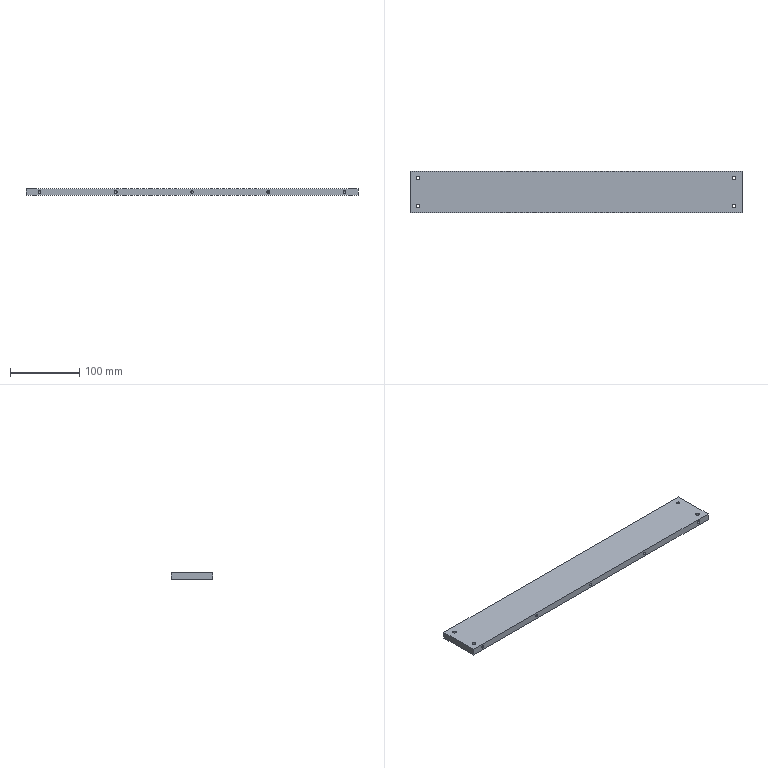Part | SolidWorks | features HoleWzd 3, Extrusion 1 | 1 solid | 46 faces | box 479 x 60 x 10 mm | volume 285459 mm3 | cylinder 24 | cone 16 | plane 6 | commonest cylinder face diameters 4.2 x10 5 x8 3.3 x6
STEP:
#1=CARTESIAN_POINT('',(0.,49.9,-1.65));
#2=VERTEX_POINT('',#1);
#3=CARTESIAN_POINT('',(0.,49.9,1.65));
#4=VERTEX_POINT('',#3);
#5=CARTESIAN_POINT('',(0.,49.9,0.));
#6=DIRECTION('',(0.,1.,0.));
#7=DIRECTION('',(0.,0.,1.));
#8=AXIS2_PLACEMENT_3D('',#5,#6,#7);
#9=CIRCLE('',#8,1.65);
#10=EDGE_CURVE('',#2,#4,#9,.T.);
#11=ORIENTED_EDGE('',*,*,#10,.F.);
#12=CARTESIAN_POINT('',(0.,60.,-1.65));
#13=VERTEX_POINT('',#12);
#14=CARTESIAN_POINT('',(0.,60.,-1.65));
#15=DIRECTION('',(0.,1.,0.));
#16=VECTOR('',#15,1000.);
#17=LINE('',#14,#16);
#18=EDGE_CURVE('',#2,#13,#17,.T.);
#19=ORIENTED_EDGE('',*,*,#18,.T.);
#20=CARTESIAN_POINT('',(0.,60.,1.65));
#21=VERTEX_POINT('',#20);
#22=CARTESIAN_POINT('',(0.,60.,0.));
#23=DIRECTION('',(0.,1.,0.));
#24=DIRECTION('',(0.,0.,1.));
#25=AXIS2_PLACEMENT_3D('',#22,#23,#24);
#26=CIRCLE('',#25,1.65);
#27=EDGE_CURVE('',#13,#21,#26,.T.);
#28=ORIENTED_EDGE('',*,*,#27,.T.);
#29=CARTESIAN_POINT('',(0.,60.,1.65));
#30=DIRECTION('',(0.,1.,0.));
#31=VECTOR('',#30,1000.);
#32=LINE('',#29,#31);
#33=EDGE_CURVE('',#4,#21,#32,.T.);
#34=ORIENTED_EDGE('',*,*,#33,.F.);
#35=EDGE_LOOP('',(#11,#19,#28,#34));
#36=FACE_OUTER_BOUND('',#35,.T.);
#37=CARTESIAN_POINT('',(0.,60.,0.));
#38=DIRECTION('',(0.,1.,0.));
#39=DIRECTION('',(0.,0.,1.));
#40=AXIS2_PLACEMENT_3D('',#37,#38,#39);
#41=CYLINDRICAL_SURFACE('',#40,1.65);
#42=ADVANCED_FACE('',(#36),#41,.F.);
#43=CARTESIAN_POINT('',(0.,48.909,0.));
#44=VERTEX_POINT('',#43);
#45=CARTESIAN_POINT('',(0.,49.9,1.65));
#46=DIRECTION('',(0.,0.515,0.8572));
#47=VECTOR('',#46,1000.);
#48=LINE('',#45,#47);
#49=EDGE_CURVE('',#44,#4,#48,.T.);
#50=ORIENTED_EDGE('',*,*,#49,.F.);
#51=CARTESIAN_POINT('',(0.,49.9,-1.65));
#52=DIRECTION('',(0.,0.515,-0.8572));
#53=VECTOR('',#52,1000.);
#54=LINE('',#51,#53);
#55=EDGE_CURVE('',#44,#2,#54,.T.);
#56=ORIENTED_EDGE('',*,*,#55,.T.);
#57=ORIENTED_EDGE('',*,*,#10,.T.);
#58=EDGE_LOOP('',(#50,#56,#57));
#59=FACE_OUTER_BOUND('',#58,.T.);
#60=CARTESIAN_POINT('',(0.,49.9,0.));
#61=DIRECTION('',(0.,1.,0.));
#62=DIRECTION('',(0.,0.,1.));
#63=AXIS2_PLACEMENT_3D('',#60,#61,#62);
#64=CONICAL_SURFACE('',#63,1.65,1.03);
#65=ADVANCED_FACE('',(#59),#64,.F.);
#66=CARTESIAN_POINT('',(-160.,49.9,-1.65));
#67=VERTEX_POINT('',#66);
#68=CARTESIAN_POINT('',(-160.,49.9,1.65));
#69=VERTEX_POINT('',#68);
#70=CARTESIAN_POINT('',(-160.,49.9,0.));
#71=DIRECTION('',(0.,1.,0.));
#72=DIRECTION('',(0.,0.,1.));
#73=AXIS2_PLACEMENT_3D('',#70,#71,#72);
#74=CIRCLE('',#73,1.65);
#75=EDGE_CURVE('',#67,#69,#74,.T.);
#76=ORIENTED_EDGE('',*,*,#75,.F.);
#77=CARTESIAN_POINT('',(-160.,60.,-1.65));
#78=VERTEX_POINT('',#77);
#79=CARTESIAN_POINT('',(-160.,60.,-1.65));
#80=DIRECTION('',(0.,1.,0.));
#81=VECTOR('',#80,1000.);
#82=LINE('',#79,#81);
#83=EDGE_CURVE('',#67,#78,#82,.T.);
#84=ORIENTED_EDGE('',*,*,#83,.T.);
#85=CARTESIAN_POINT('',(-160.,60.,1.65));
#86=VERTEX_POINT('',#85);
#87=CARTESIAN_POINT('',(-160.,60.,0.));
#88=DIRECTION('',(0.,1.,0.));
#89=DIRECTION('',(0.,0.,1.));
#90=AXIS2_PLACEMENT_3D('',#87,#88,#89);
#91=CIRCLE('',#90,1.65);
#92=EDGE_CURVE('',#78,#86,#91,.T.);
#93=ORIENTED_EDGE('',*,*,#92,.T.);
#94=CARTESIAN_POINT('',(-160.,60.,1.65));
#95=DIRECTION('',(0.,1.,0.));
#96=VECTOR('',#95,1000.);
#97=LINE('',#94,#96);
#98=EDGE_CURVE('',#69,#86,#97,.T.);
#99=ORIENTED_EDGE('',*,*,#98,.F.);
#100=EDGE_LOOP('',(#76,#84,#93,#99));
#101=FACE_OUTER_BOUND('',#100,.T.);
#102=CARTESIAN_POINT('',(-160.,60.,0.));
#103=DIRECTION('',(0.,1.,0.));
#104=DIRECTION('',(0.,0.,1.));
#105=AXIS2_PLACEMENT_3D('',#102,#103,#104);
#106=CYLINDRICAL_SURFACE('',#105,1.65);
#107=ADVANCED_FACE('',(#101),#106,.F.);
#108=CARTESIAN_POINT('',(-160.,48.909,0.));
#109=VERTEX_POINT('',#108);
#110=CARTESIAN_POINT('',(-160.,49.9,1.65));
#111=DIRECTION('',(0.,0.515,0.8572));
#112=VECTOR('',#111,1000.);
#113=LINE('',#110,#112);
#114=EDGE_CURVE('',#109,#69,#113,.T.);
#115=ORIENTED_EDGE('',*,*,#114,.F.);
#116=CARTESIAN_POINT('',(-160.,49.9,-1.65));
#117=DIRECTION('',(0.,0.515,-0.8572));
#118=VECTOR('',#117,1000.);
#119=LINE('',#116,#118);
#120=EDGE_CURVE('',#109,#67,#119,.T.);
#121=ORIENTED_EDGE('',*,*,#120,.T.);
#122=ORIENTED_EDGE('',*,*,#75,.T.);
#123=EDGE_LOOP('',(#115,#121,#122));
#124=FACE_OUTER_BOUND('',#123,.T.);
#125=CARTESIAN_POINT('',(-160.,49.9,0.));
#126=DIRECTION('',(0.,1.,0.));
#127=DIRECTION('',(0.,0.,1.));
#128=AXIS2_PLACEMENT_3D('',#125,#126,#127);
#129=CONICAL_SURFACE('',#128,1.65,1.03);
#130=ADVANCED_FACE('',(#124),#129,.F.);
#131=CARTESIAN_POINT('',(160.,49.9,-1.65));
#132=VERTEX_POINT('',#131);
#133=CARTESIAN_POINT('',(160.,49.9,1.65));
#134=VERTEX_POINT('',#133);
#135=CARTESIAN_POINT('',(160.,49.9,0.));
#136=DIRECTION('',(0.,1.,0.));
#137=DIRECTION('',(0.,0.,1.));
#138=AXIS2_PLACEMENT_3D('',#135,#136,#137);
#139=CIRCLE('',#138,1.65);
#140=EDGE_CURVE('',#132,#134,#139,.T.);
#141=ORIENTED_EDGE('',*,*,#140,.F.);
#142=CARTESIAN_POINT('',(160.,60.,-1.65));
#143=VERTEX_POINT('',#142);
#144=CARTESIAN_POINT('',(160.,60.,-1.65));
#145=DIRECTION('',(0.,1.,0.));
#146=VECTOR('',#145,1000.);
#147=LINE('',#144,#146);
#148=EDGE_CURVE('',#132,#143,#147,.T.);
#149=ORIENTED_EDGE('',*,*,#148,.T.);
#150=CARTESIAN_POINT('',(160.,60.,1.65));
#151=VERTEX_POINT('',#150);
#152=CARTESIAN_POINT('',(160.,60.,0.));
#153=DIRECTION('',(0.,1.,0.));
#154=DIRECTION('',(0.,0.,1.));
#155=AXIS2_PLACEMENT_3D('',#152,#153,#154);
#156=CIRCLE('',#155,1.65);
#157=EDGE_CURVE('',#143,#151,#156,.T.);
#158=ORIENTED_EDGE('',*,*,#157,.T.);
#159=CARTESIAN_POINT('',(160.,60.,1.65));
#160=DIRECTION('',(0.,1.,0.));
#161=VECTOR('',#160,1000.);
#162=LINE('',#159,#161);
#163=EDGE_CURVE('',#134,#151,#162,.T.);
#164=ORIENTED_EDGE('',*,*,#163,.F.);
#165=EDGE_LOOP('',(#141,#149,#158,#164));
#166=FACE_OUTER_BOUND('',#165,.T.);
#167=CARTESIAN_POINT('',(160.,60.,0.));
#168=DIRECTION('',(0.,1.,0.));
#169=DIRECTION('',(0.,0.,1.));
#170=AXIS2_PLACEMENT_3D('',#167,#168,#169);
#171=CYLINDRICAL_SURFACE('',#170,1.65);
#172=ADVANCED_FACE('',(#166),#171,.F.);
#173=CARTESIAN_POINT('',(160.,48.909,0.));
#174=VERTEX_POINT('',#173);
#175=CARTESIAN_POINT('',(160.,49.9,1.65));
#176=DIRECTION('',(0.,0.515,0.8572));
#177=VECTOR('',#176,1000.);
#178=LINE('',#175,#177);
#179=EDGE_CURVE('',#174,#134,#178,.T.);
#180=ORIENTED_EDGE('',*,*,#179,.F.);
#181=CARTESIAN_POINT('',(160.,49.9,-1.65));
#182=DIRECTION('',(0.,0.515,-0.8572));
#183=VECTOR('',#182,1000.);
#184=LINE('',#181,#183);
#185=EDGE_CURVE('',#174,#132,#184,.T.);
#186=ORIENTED_EDGE('',*,*,#185,.T.);
#187=ORIENTED_EDGE('',*,*,#140,.T.);
#188=EDGE_LOOP('',(#180,#186,#187));
#189=FACE_OUTER_BOUND('',#188,.T.);
#190=CARTESIAN_POINT('',(160.,49.9,0.));
#191=DIRECTION('',(0.,1.,0.));
#192=DIRECTION('',(0.,0.,1.));
#193=AXIS2_PLACEMENT_3D('',#190,#191,#192);
#194=CONICAL_SURFACE('',#193,1.65,1.03);
#195=ADVANCED_FACE('',(#189),#194,.F.);
#196=CARTESIAN_POINT('',(-225.5,50.,5.));
#197=VERTEX_POINT('',#196);
#198=CARTESIAN_POINT('',(-230.5,50.,5.));
#199=VERTEX_POINT('',#198);
#200=CARTESIAN_POINT('',(-228.,50.,5.));
#201=DIRECTION('',(0.,0.,-1.));
#202=DIRECTION('',(-1.,0.,0.));
#203=AXIS2_PLACEMENT_3D('',#200,#201,#202);
#204=CIRCLE('',#203,2.5);
#205=EDGE_CURVE('',#197,#199,#204,.T.);
#206=ORIENTED_EDGE('',*,*,#205,.F.);
#207=CARTESIAN_POINT('',(-225.5,50.,-5.));
#208=VERTEX_POINT('',#207);
#209=CARTESIAN_POINT('',(-225.5,50.,-5.));
#210=DIRECTION('',(0.,0.,-1.));
#211=VECTOR('',#210,1000.);
#212=LINE('',#209,#211);
#213=EDGE_CURVE('',#197,#208,#212,.T.);
#214=ORIENTED_EDGE('',*,*,#213,.T.);
#215=CARTESIAN_POINT('',(-230.5,50.,-5.));
#216=VERTEX_POINT('',#215);
#217=CARTESIAN_POINT('',(-228.,50.,-5.));
#218=DIRECTION('',(0.,0.,-1.));
#219=DIRECTION('',(-1.,0.,0.));
#220=AXIS2_PLACEMENT_3D('',#217,#218,#219);
#221=CIRCLE('',#220,2.5);
#222=EDGE_CURVE('',#208,#216,#221,.T.);
#223=ORIENTED_EDGE('',*,*,#222,.T.);
#224=CARTESIAN_POINT('',(-230.5,50.,-5.));
#225=DIRECTION('',(0.,0.,-1.));
#226=VECTOR('',#225,1000.);
#227=LINE('',#224,#226);
#228=EDGE_CURVE('',#199,#216,#227,.T.);
#229=ORIENTED_EDGE('',*,*,#228,.F.);
#230=EDGE_LOOP('',(#206,#214,#223,#229));
#231=FACE_OUTER_BOUND('',#230,.T.);
#232=CARTESIAN_POINT('',(-228.,50.,-5.));
#233=DIRECTION('',(0.,0.,-1.));
#234=DIRECTION('',(-1.,0.,0.));
#235=AXIS2_PLACEMENT_3D('',#232,#233,#234);
#236=CYLINDRICAL_SURFACE('',#235,2.5);
#237=ADVANCED_FACE('',(#231),#236,.F.);
#238=CARTESIAN_POINT('',(-225.5,10.,5.));
#239=VERTEX_POINT('',#238);
#240=CARTESIAN_POINT('',(-230.5,10.,5.));
#241=VERTEX_POINT('',#240);
#242=CARTESIAN_POINT('',(-228.,10.,5.));
#243=DIRECTION('',(0.,0.,-1.));
#244=DIRECTION('',(-1.,0.,0.));
#245=AXIS2_PLACEMENT_3D('',#242,#243,#244);
#246=CIRCLE('',#245,2.5);
#247=EDGE_CURVE('',#239,#241,#246,.T.);
#248=ORIENTED_EDGE('',*,*,#247,.F.);
#249=CARTESIAN_POINT('',(-225.5,10.,-5.));
#250=VERTEX_POINT('',#249);
#251=CARTESIAN_POINT('',(-225.5,10.,-5.));
#252=DIRECTION('',(0.,0.,-1.));
#253=VECTOR('',#252,1000.);
#254=LINE('',#251,#253);
#255=EDGE_CURVE('',#239,#250,#254,.T.);
#256=ORIENTED_EDGE('',*,*,#255,.T.);
#257=CARTESIAN_POINT('',(-230.5,10.,-5.));
#258=VERTEX_POINT('',#257);
#259=CARTESIAN_POINT('',(-228.,10.,-5.));
#260=DIRECTION('',(0.,0.,-1.));
#261=DIRECTION('',(-1.,0.,0.));
#262=AXIS2_PLACEMENT_3D('',#259,#260,#261);
#263=CIRCLE('',#262,2.5);
#264=EDGE_CURVE('',#250,#258,#263,.T.);
#265=ORIENTED_EDGE('',*,*,#264,.T.);
#266=CARTESIAN_POINT('',(-230.5,10.,-5.));
#267=DIRECTION('',(0.,0.,-1.));
#268=VECTOR('',#267,1000.);
#269=LINE('',#266,#268);
#270=EDGE_CURVE('',#241,#258,#269,.T.);
#271=ORIENTED_EDGE('',*,*,#270,.F.);
#272=EDGE_LOOP('',(#248,#256,#265,#271));
#273=FACE_OUTER_BOUND('',#272,.T.);
#274=CARTESIAN_POINT('',(-228.,10.,-5.));
#275=DIRECTION('',(0.,0.,-1.));
#276=DIRECTION('',(-1.,0.,0.));
#277=AXIS2_PLACEMENT_3D('',#274,#275,#276);
#278=CYLINDRICAL_SURFACE('',#277,2.5);
#279=ADVANCED_FACE('',(#273),#278,.F.);
#280=CARTESIAN_POINT('',(230.5,10.,5.));
#281=VERTEX_POINT('',#280);
#282=CARTESIAN_POINT('',(225.5,10.,5.));
#283=VERTEX_POINT('',#282);
#284=CARTESIAN_POINT('',(228.,10.,5.));
#285=DIRECTION('',(0.,0.,-1.));
#286=DIRECTION('',(-1.,0.,0.));
#287=AXIS2_PLACEMENT_3D('',#284,#285,#286);
#288=CIRCLE('',#287,2.5);
#289=EDGE_CURVE('',#281,#283,#288,.T.);
#290=ORIENTED_EDGE('',*,*,#289,.F.);
#291=CARTESIAN_POINT('',(230.5,10.,-5.));
#292=VERTEX_POINT('',#291);
#293=CARTESIAN_POINT('',(230.5,10.,-5.));
#294=DIRECTION('',(0.,0.,-1.));
#295=VECTOR('',#294,1000.);
#296=LINE('',#293,#295);
#297=EDGE_CURVE('',#281,#292,#296,.T.);
#298=ORIENTED_EDGE('',*,*,#297,.T.);
#299=CARTESIAN_POINT('',(225.5,10.,-5.));
#300=VERTEX_POINT('',#299);
#301=CARTESIAN_POINT('',(228.,10.,-5.));
#302=DIRECTION('',(0.,0.,-1.));
#303=DIRECTION('',(-1.,0.,0.));
#304=AXIS2_PLACEMENT_3D('',#301,#302,#303);
#305=CIRCLE('',#304,2.5);
#306=EDGE_CURVE('',#292,#300,#305,.T.);
#307=ORIENTED_EDGE('',*,*,#306,.T.);
#308=CARTESIAN_POINT('',(225.5,10.,-5.));
#309=DIRECTION('',(0.,0.,-1.));
#310=VECTOR('',#309,1000.);
#311=LINE('',#308,#310);
#312=EDGE_CURVE('',#283,#300,#311,.T.);
#313=ORIENTED_EDGE('',*,*,#312,.F.);
#314=EDGE_LOOP('',(#290,#298,#307,#313));
#315=FACE_OUTER_BOUND('',#314,.T.);
#316=CARTESIAN_POINT('',(228.,10.,-5.));
#317=DIRECTION('',(0.,0.,-1.));
#318=DIRECTION('',(-1.,0.,0.));
#319=AXIS2_PLACEMENT_3D('',#316,#317,#318);
#320=CYLINDRICAL_SURFACE('',#319,2.5);
#321=ADVANCED_FACE('',(#315),#320,.F.);
#322=CARTESIAN_POINT('',(230.5,50.,5.));
#323=VERTEX_POINT('',#322);
#324=CARTESIAN_POINT('',(225.5,50.,5.));
#325=VERTEX_POINT('',#324);
#326=CARTESIAN_POINT('',(228.,50.,5.));
#327=DIRECTION('',(0.,0.,-1.));
#328=DIRECTION('',(-1.,0.,0.));
#329=AXIS2_PLACEMENT_3D('',#326,#327,#328);
#330=CIRCLE('',#329,2.5);
#331=EDGE_CURVE('',#323,#325,#330,.T.);
#332=ORIENTED_EDGE('',*,*,#331,.F.);
#333=CARTESIAN_POINT('',(230.5,50.,-5.));
#334=VERTEX_POINT('',#333);
#335=CARTESIAN_POINT('',(230.5,50.,-5.));
#336=DIRECTION('',(0.,0.,-1.));
#337=VECTOR('',#336,1000.);
#338=LINE('',#335,#337);
#339=EDGE_CURVE('',#323,#334,#338,.T.);
#340=ORIENTED_EDGE('',*,*,#339,.T.);
#341=CARTESIAN_POINT('',(225.5,50.,-5.));
#342=VERTEX_POINT('',#341);
#343=CARTESIAN_POINT('',(228.,50.,-5.));
#344=DIRECTION('',(0.,0.,-1.));
#345=DIRECTION('',(-1.,0.,0.));
#346=AXIS2_PLACEMENT_3D('',#343,#344,#345);
#347=CIRCLE('',#346,2.5);
#348=EDGE_CURVE('',#334,#342,#347,.T.);
#349=ORIENTED_EDGE('',*,*,#348,.T.);
#350=CARTESIAN_POINT('',(225.5,50.,-5.));
#351=DIRECTION('',(0.,0.,-1.));
#352=VECTOR('',#351,1000.);
#353=LINE('',#350,#352);
#354=EDGE_CURVE('',#325,#342,#353,.T.);
#355=ORIENTED_EDGE('',*,*,#354,.F.);
#356=EDGE_LOOP('',(#332,#340,#349,#355));
#357=FACE_OUTER_BOUND('',#356,.T.);
#358=CARTESIAN_POINT('',(228.,50.,-5.));
#359=DIRECTION('',(0.,0.,-1.));
#360=DIRECTION('',(-1.,0.,0.));
#361=AXIS2_PLACEMENT_3D('',#358,#359,#360);
#362=CYLINDRICAL_SURFACE('',#361,2.5);
#363=ADVANCED_FACE('',(#357),#362,.F.);
#364=CARTESIAN_POINT('',(0.,12.4,2.1));
#365=VERTEX_POINT('',#364);
#366=CARTESIAN_POINT('',(0.,12.4,-2.1));
#367=VERTEX_POINT('',#366);
#368=CARTESIAN_POINT('',(0.,12.4,0.));
#369=DIRECTION('',(0.,-1.,0.));
#370=DIRECTION('',(0.,0.,-1.));
#371=AXIS2_PLACEMENT_3D('',#368,#369,#370);
#372=CIRCLE('',#371,2.1);
#373=EDGE_CURVE('',#365,#367,#372,.T.);
#374=ORIENTED_EDGE('',*,*,#373,.F.);
#375=CARTESIAN_POINT('',(0.,0.,2.1));
#376=VERTEX_POINT('',#375);
#377=CARTESIAN_POINT('',(0.,0.,2.1));
#378=DIRECTION('',(0.,-1.,0.));
#379=VECTOR('',#378,1000.);
#380=LINE('',#377,#379);
#381=EDGE_CURVE('',#365,#376,#380,.T.);
#382=ORIENTED_EDGE('',*,*,#381,.T.);
#383=CARTESIAN_POINT('',(0.,0.,-2.1));
#384=VERTEX_POINT('',#383);
#385=CARTESIAN_POINT('',(0.,0.,0.));
#386=DIRECTION('',(0.,-1.,0.));
#387=DIRECTION('',(0.,0.,-1.));
#388=AXIS2_PLACEMENT_3D('',#385,#386,#387);
#389=CIRCLE('',#388,2.1);
#390=EDGE_CURVE('',#376,#384,#389,.T.);
#391=ORIENTED_EDGE('',*,*,#390,.T.);
#392=CARTESIAN_POINT('',(0.,0.,-2.1));
#393=DIRECTION('',(0.,-1.,0.));
#394=VECTOR('',#393,1000.);
#395=LINE('',#392,#394);
#396=EDGE_CURVE('',#367,#384,#395,.T.);
#397=ORIENTED_EDGE('',*,*,#396,.F.);
#398=EDGE_LOOP('',(#374,#382,#391,#397));
#399=FACE_OUTER_BOUND('',#398,.T.);
#400=CARTESIAN_POINT('',(0.,0.,0.));
#401=DIRECTION('',(0.,-1.,0.));
#402=DIRECTION('',(0.,0.,-1.));
#403=AXIS2_PLACEMENT_3D('',#400,#401,#402);
#404=CYLINDRICAL_SURFACE('',#403,2.1);
#405=ADVANCED_FACE('',(#399),#404,.F.);
#406=CARTESIAN_POINT('',(0.,13.662,0.));
#407=VERTEX_POINT('',#406);
#408=CARTESIAN_POINT('',(0.,12.4,-2.1));
#409=DIRECTION('',(0.,-0.515,-0.8572));
#410=VECTOR('',#409,1000.);
#411=LINE('',#408,#410);
#412=EDGE_CURVE('',#407,#367,#411,.T.);
#413=ORIENTED_EDGE('',*,*,#412,.F.);
#414=CARTESIAN_POINT('',(0.,12.4,2.1));
#415=DIRECTION('',(0.,-0.515,0.8572));
#416=VECTOR('',#415,1000.);
#417=LINE('',#414,#416);
#418=EDGE_CURVE('',#407,#365,#417,.T.);
#419=ORIENTED_EDGE('',*,*,#418,.T.);
#420=ORIENTED_EDGE('',*,*,#373,.T.);
#421=EDGE_LOOP('',(#413,#419,#420));
#422=FACE_OUTER_BOUND('',#421,.T.);
#423=CARTESIAN_POINT('',(0.,12.4,0.));
#424=DIRECTION('',(0.,-1.,0.));
#425=DIRECTION('',(0.,0.,-1.));
#426=AXIS2_PLACEMENT_3D('',#423,#424,#425);
#427=CONICAL_SURFACE('',#426,2.1,1.03);
#428=ADVANCED_FACE('',(#422),#427,.F.);
#429=CARTESIAN_POINT('',(110.,12.4,2.1));
#430=VERTEX_POINT('',#429);
#431=CARTESIAN_POINT('',(110.,12.4,-2.1));
#432=VERTEX_POINT('',#431);
#433=CARTESIAN_POINT('',(110.,12.4,0.));
#434=DIRECTION('',(0.,-1.,0.));
#435=DIRECTION('',(0.,0.,-1.));
#436=AXIS2_PLACEMENT_3D('',#433,#434,#435);
#437=CIRCLE('',#436,2.1);
#438=EDGE_CURVE('',#430,#432,#437,.T.);
#439=ORIENTED_EDGE('',*,*,#438,.F.);
#440=CARTESIAN_POINT('',(110.,0.,2.1));
#441=VERTEX_POINT('',#440);
#442=CARTESIAN_POINT('',(110.,0.,2.1));
#443=DIRECTION('',(0.,-1.,0.));
#444=VECTOR('',#443,1000.);
#445=LINE('',#442,#444);
#446=EDGE_CURVE('',#430,#441,#445,.T.);
#447=ORIENTED_EDGE('',*,*,#446,.T.);
#448=CARTESIAN_POINT('',(110.,0.,-2.1));
#449=VERTEX_POINT('',#448);
#450=CARTESIAN_POINT('',(110.,0.,0.));
#451=DIRECTION('',(0.,-1.,0.));
#452=DIRECTION('',(0.,0.,-1.));
#453=AXIS2_PLACEMENT_3D('',#450,#451,#452);
#454=CIRCLE('',#453,2.1);
#455=EDGE_CURVE('',#441,#449,#454,.T.);
#456=ORIENTED_EDGE('',*,*,#455,.T.);
#457=CARTESIAN_POINT('',(110.,0.,-2.1));
#458=DIRECTION('',(0.,-1.,0.));
#459=VECTOR('',#458,1000.);
#460=LINE('',#457,#459);
#461=EDGE_CURVE('',#432,#449,#460,.T.);
#462=ORIENTED_EDGE('',*,*,#461,.F.);
#463=EDGE_LOOP('',(#439,#447,#456,#462));
#464=FACE_OUTER_BOUND('',#463,.T.);
#465=CARTESIAN_POINT('',(110.,0.,0.));
#466=DIRECTION('',(0.,-1.,0.));
#467=DIRECTION('',(0.,0.,-1.));
#468=AXIS2_PLACEMENT_3D('',#465,#466,#467);
#469=CYLINDRICAL_SURFACE('',#468,2.1);
#470=ADVANCED_FACE('',(#464),#469,.F.);
#471=CARTESIAN_POINT('',(110.,13.662,0.));
#472=VERTEX_POINT('',#471);
#473=CARTESIAN_POINT('',(110.,12.4,-2.1));
#474=DIRECTION('',(0.,-0.515,-0.8572));
#475=VECTOR('',#474,1000.);
#476=LINE('',#473,#475);
#477=EDGE_CURVE('',#472,#432,#476,.T.);
#478=ORIENTED_EDGE('',*,*,#477,.F.);
#479=CARTESIAN_POINT('',(110.,12.4,2.1));
#480=DIRECTION('',(0.,-0.515,0.8572));
#481=VECTOR('',#480,1000.);
#482=LINE('',#479,#481);
#483=EDGE_CURVE('',#472,#430,#482,.T.);
#484=ORIENTED_EDGE('',*,*,#483,.T.);
#485=ORIENTED_EDGE('',*,*,#438,.T.);
#486=EDGE_LOOP('',(#478,#484,#485));
#487=FACE_OUTER_BOUND('',#486,.T.);
#488=CARTESIAN_POINT('',(110.,12.4,0.));
#489=DIRECTION('',(0.,-1.,0.));
#490=DIRECTION('',(0.,0.,-1.));
#491=AXIS2_PLACEMENT_3D('',#488,#489,#490);
#492=CONICAL_SURFACE('',#491,2.1,1.03);
#493=ADVANCED_FACE('',(#487),#492,.F.);
#494=CARTESIAN_POINT('',(220.,12.4,2.1));
#495=VERTEX_POINT('',#494);
#496=CARTESIAN_POINT('',(220.,12.4,-2.1));
#497=VERTEX_POINT('',#496);
#498=CARTESIAN_POINT('',(220.,12.4,0.));
#499=DIRECTION('',(0.,-1.,0.));
#500=DIRECTION('',(0.,0.,-1.));
#501=AXIS2_PLACEMENT_3D('',#498,#499,#500);
#502=CIRCLE('',#501,2.1);
#503=EDGE_CURVE('',#495,#497,#502,.T.);
#504=ORIENTED_EDGE('',*,*,#503,.F.);
#505=CARTESIAN_POINT('',(220.,0.,2.1));
#506=VERTEX_POINT('',#505);
#507=CARTESIAN_POINT('',(220.,0.,2.1));
#508=DIRECTION('',(0.,-1.,0.));
#509=VECTOR('',#508,1000.);
#510=LINE('',#507,#509);
#511=EDGE_CURVE('',#495,#506,#510,.T.);
#512=ORIENTED_EDGE('',*,*,#511,.T.);
#513=CARTESIAN_POINT('',(220.,0.,-2.1));
#514=VERTEX_POINT('',#513);
#515=CARTESIAN_POINT('',(220.,0.,0.));
#516=DIRECTION('',(0.,-1.,0.));
#517=DIRECTION('',(0.,0.,-1.));
#518=AXIS2_PLACEMENT_3D('',#515,#516,#517);
#519=CIRCLE('',#518,2.1);
#520=EDGE_CURVE('',#506,#514,#519,.T.);
#521=ORIENTED_EDGE('',*,*,#520,.T.);
#522=CARTESIAN_POINT('',(220.,0.,-2.1));
#523=DIRECTION('',(0.,-1.,0.));
#524=VECTOR('',#523,1000.);
#525=LINE('',#522,#524);
#526=EDGE_CURVE('',#497,#514,#525,.T.);
#527=ORIENTED_EDGE('',*,*,#526,.F.);
#528=EDGE_LOOP('',(#504,#512,#521,#527));
#529=FACE_OUTER_BOUND('',#528,.T.);
#530=CARTESIAN_POINT('',(220.,0.,0.));
#531=DIRECTION('',(0.,-1.,0.));
#532=DIRECTION('',(0.,0.,-1.));
#533=AXIS2_PLACEMENT_3D('',#530,#531,#532);
#534=CYLINDRICAL_SURFACE('',#533,2.1);
#535=ADVANCED_FACE('',(#529),#534,.F.);
#536=CARTESIAN_POINT('',(220.,13.662,0.));
#537=VERTEX_POINT('',#536);
#538=CARTESIAN_POINT('',(220.,12.4,-2.1));
#539=DIRECTION('',(0.,-0.515,-0.8572));
#540=VECTOR('',#539,1000.);
#541=LINE('',#538,#540);
#542=EDGE_CURVE('',#537,#497,#541,.T.);
#543=ORIENTED_EDGE('',*,*,#542,.F.);
#544=CARTESIAN_POINT('',(220.,12.4,2.1));
#545=DIRECTION('',(0.,-0.515,0.8572));
#546=VECTOR('',#545,1000.);
#547=LINE('',#544,#546);
#548=EDGE_CURVE('',#537,#495,#547,.T.);
#549=ORIENTED_EDGE('',*,*,#548,.T.);
#550=ORIENTED_EDGE('',*,*,#503,.T.);
#551=EDGE_LOOP('',(#543,#549,#550));
#552=FACE_OUTER_BOUND('',#551,.T.);
#553=CARTESIAN_POINT('',(220.,12.4,0.));
#554=DIRECTION('',(0.,-1.,0.));
#555=DIRECTION('',(0.,0.,-1.));
#556=AXIS2_PLACEMENT_3D('',#553,#554,#555);
#557=CONICAL_SURFACE('',#556,2.1,1.03);
#558=ADVANCED_FACE('',(#552),#557,.F.);
#559=CARTESIAN_POINT('',(-220.,12.4,2.1));
#560=VERTEX_POINT('',#559);
#561=CARTESIAN_POINT('',(-220.,12.4,-2.1));
#562=VERTEX_POINT('',#561);
#563=CARTESIAN_POINT('',(-220.,12.4,0.));
#564=DIRECTION('',(0.,-1.,0.));
#565=DIRECTION('',(0.,0.,-1.));
#566=AXIS2_PLACEMENT_3D('',#563,#564,#565);
#567=CIRCLE('',#566,2.1);
#568=EDGE_CURVE('',#560,#562,#567,.T.);
#569=ORIENTED_EDGE('',*,*,#568,.F.);
#570=CARTESIAN_POINT('',(-220.,0.,2.1));
#571=VERTEX_POINT('',#570);
#572=CARTESIAN_POINT('',(-220.,0.,2.1));
#573=DIRECTION('',(0.,-1.,0.));
#574=VECTOR('',#573,1000.);
#575=LINE('',#572,#574);
#576=EDGE_CURVE('',#560,#571,#575,.T.);
#577=ORIENTED_EDGE('',*,*,#576,.T.);
#578=CARTESIAN_POINT('',(-220.,0.,-2.1));
#579=VERTEX_POINT('',#578);
#580=CARTESIAN_POINT('',(-220.,0.,0.));
#581=DIRECTION('',(0.,-1.,0.));
#582=DIRECTION('',(0.,0.,-1.));
#583=AXIS2_PLACEMENT_3D('',#580,#581,#582);
#584=CIRCLE('',#583,2.1);
#585=EDGE_CURVE('',#571,#579,#584,.T.);
#586=ORIENTED_EDGE('',*,*,#585,.T.);
#587=CARTESIAN_POINT('',(-220.,0.,-2.1));
#588=DIRECTION('',(0.,-1.,0.));
#589=VECTOR('',#588,1000.);
#590=LINE('',#587,#589);
#591=EDGE_CURVE('',#562,#579,#590,.T.);
#592=ORIENTED_EDGE('',*,*,#591,.F.);
#593=EDGE_LOOP('',(#569,#577,#586,#592));
#594=FACE_OUTER_BOUND('',#593,.T.);
#595=CARTESIAN_POINT('',(-220.,0.,0.));
#596=DIRECTION('',(0.,-1.,0.));
#597=DIRECTION('',(0.,0.,-1.));
#598=AXIS2_PLACEMENT_3D('',#595,#596,#597);
#599=CYLINDRICAL_SURFACE('',#598,2.1);
#600=ADVANCED_FACE('',(#594),#599,.F.);
#601=CARTESIAN_POINT('',(-220.,13.662,0.));
#602=VERTEX_POINT('',#601);
#603=CARTESIAN_POINT('',(-220.,12.4,-2.1));
#604=DIRECTION('',(0.,-0.515,-0.8572));
#605=VECTOR('',#604,1000.);
#606=LINE('',#603,#605);
#607=EDGE_CURVE('',#602,#562,#606,.T.);
#608=ORIENTED_EDGE('',*,*,#607,.F.);
#609=CARTESIAN_POINT('',(-220.,12.4,2.1));
#610=DIRECTION('',(0.,-0.515,0.8572));
#611=VECTOR('',#610,1000.);
#612=LINE('',#609,#611);
#613=EDGE_CURVE('',#602,#560,#612,.T.);
#614=ORIENTED_EDGE('',*,*,#613,.T.);
#615=ORIENTED_EDGE('',*,*,#568,.T.);
#616=EDGE_LOOP('',(#608,#614,#615));
#617=FACE_OUTER_BOUND('',#616,.T.);
#618=CARTESIAN_POINT('',(-220.,12.4,0.));
#619=DIRECTION('',(0.,-1.,0.));
#620=DIRECTION('',(0.,0.,-1.));
#621=AXIS2_PLACEMENT_3D('',#618,#619,#620);
#622=CONICAL_SURFACE('',#621,2.1,1.03);
#623=ADVANCED_FACE('',(#617),#622,.F.);
#624=CARTESIAN_POINT('',(-110.,12.4,2.1));
#625=VERTEX_POINT('',#624);
#626=CARTESIAN_POINT('',(-110.,12.4,-2.1));
#627=VERTEX_POINT('',#626);
#628=CARTESIAN_POINT('',(-110.,12.4,0.));
#629=DIRECTION('',(0.,-1.,0.));
#630=DIRECTION('',(0.,0.,-1.));
#631=AXIS2_PLACEMENT_3D('',#628,#629,#630);
#632=CIRCLE('',#631,2.1);
#633=EDGE_CURVE('',#625,#627,#632,.T.);
#634=ORIENTED_EDGE('',*,*,#633,.F.);
#635=CARTESIAN_POINT('',(-110.,0.,2.1));
#636=VERTEX_POINT('',#635);
#637=CARTESIAN_POINT('',(-110.,0.,2.1));
#638=DIRECTION('',(0.,-1.,0.));
#639=VECTOR('',#638,1000.);
#640=LINE('',#637,#639);
#641=EDGE_CURVE('',#625,#636,#640,.T.);
#642=ORIENTED_EDGE('',*,*,#641,.T.);
#643=CARTESIAN_POINT('',(-110.,0.,-2.1));
#644=VERTEX_POINT('',#643);
#645=CARTESIAN_POINT('',(-110.,0.,0.));
#646=DIRECTION('',(0.,-1.,0.));
#647=DIRECTION('',(0.,0.,-1.));
#648=AXIS2_PLACEMENT_3D('',#645,#646,#647);
#649=CIRCLE('',#648,2.1);
#650=EDGE_CURVE('',#636,#644,#649,.T.);
#651=ORIENTED_EDGE('',*,*,#650,.T.);
#652=CARTESIAN_POINT('',(-110.,0.,-2.1));
#653=DIRECTION('',(0.,-1.,0.));
#654=VECTOR('',#653,1000.);
#655=LINE('',#652,#654);
#656=EDGE_CURVE('',#627,#644,#655,.T.);
#657=ORIENTED_EDGE('',*,*,#656,.F.);
#658=EDGE_LOOP('',(#634,#642,#651,#657));
#659=FACE_OUTER_BOUND('',#658,.T.);
#660=CARTESIAN_POINT('',(-110.,0.,0.));
#661=DIRECTION('',(0.,-1.,0.));
#662=DIRECTION('',(0.,0.,-1.));
#663=AXIS2_PLACEMENT_3D('',#660,#661,#662);
#664=CYLINDRICAL_SURFACE('',#663,2.1);
#665=ADVANCED_FACE('',(#659),#664,.F.);
#666=CARTESIAN_POINT('',(-110.,13.662,0.));
#667=VERTEX_POINT('',#666);
#668=CARTESIAN_POINT('',(-110.,12.4,-2.1));
#669=DIRECTION('',(0.,-0.515,-0.8572));
#670=VECTOR('',#669,1000.);
#671=LINE('',#668,#670);
#672=EDGE_CURVE('',#667,#627,#671,.T.);
#673=ORIENTED_EDGE('',*,*,#672,.F.);
#674=CARTESIAN_POINT('',(-110.,12.4,2.1));
#675=DIRECTION('',(0.,-0.515,0.8572));
#676=VECTOR('',#675,1000.);
#677=LINE('',#674,#676);
#678=EDGE_CURVE('',#667,#625,#677,.T.);
#679=ORIENTED_EDGE('',*,*,#678,.T.);
#680=ORIENTED_EDGE('',*,*,#633,.T.);
#681=EDGE_LOOP('',(#673,#679,#680));
#682=FACE_OUTER_BOUND('',#681,.T.);
#683=CARTESIAN_POINT('',(-110.,12.4,0.));
#684=DIRECTION('',(0.,-1.,0.));
#685=DIRECTION('',(0.,0.,-1.));
#686=AXIS2_PLACEMENT_3D('',#683,#684,#685);
#687=CONICAL_SURFACE('',#686,2.1,1.03);
#688=ADVANCED_FACE('',(#682),#687,.F.);
#689=CARTESIAN_POINT('',(239.5,0.,5.));
#690=VERTEX_POINT('',#689);
#691=CARTESIAN_POINT('',(239.5,0.,-5.));
#692=VERTEX_POINT('',#691);
#693=CARTESIAN_POINT('',(239.5,0.,5.));
#694=DIRECTION('',(0.,0.,-1.));
#695=VECTOR('',#694,1000.);
#696=LINE('',#693,#695);
#697=EDGE_CURVE('',#690,#692,#696,.T.);
#698=ORIENTED_EDGE('',*,*,#697,.T.);
#699=CARTESIAN_POINT('',(239.5,60.,-5.));
#700=VERTEX_POINT('',#699);
#701=CARTESIAN_POINT('',(239.5,60.,-5.));
#702=DIRECTION('',(0.,-1.,0.));
#703=VECTOR('',#702,1000.);
#704=LINE('',#701,#703);
#705=EDGE_CURVE('',#700,#692,#704,.T.);
#706=ORIENTED_EDGE('',*,*,#705,.F.);
#707=CARTESIAN_POINT('',(239.5,60.,5.));
#708=VERTEX_POINT('',#707);
#709=CARTESIAN_POINT('',(239.5,60.,5.));
#710=DIRECTION('',(0.,0.,-1.));
#711=VECTOR('',#710,1000.);
#712=LINE('',#709,#711);
#713=EDGE_CURVE('',#708,#700,#712,.T.);
#714=ORIENTED_EDGE('',*,*,#713,.F.);
#715=CARTESIAN_POINT('',(239.5,60.,5.));
#716=DIRECTION('',(0.,-1.,0.));
#717=VECTOR('',#716,1000.);
#718=LINE('',#715,#717);
#719=EDGE_CURVE('',#708,#690,#718,.T.);
#720=ORIENTED_EDGE('',*,*,#719,.T.);
#721=EDGE_LOOP('',(#698,#706,#714,#720));
#722=FACE_OUTER_BOUND('',#721,.T.);
#723=CARTESIAN_POINT('',(239.5,60.,5.));
#724=DIRECTION('',(-1.,0.,0.));
#725=DIRECTION('',(0.,0.,1.));
#726=AXIS2_PLACEMENT_3D('',#723,#724,#725);
#727=PLANE('',#726);
#728=ADVANCED_FACE('',(#722),#727,.F.);
#729=CARTESIAN_POINT('',(-228.,50.,-5.));
#730=DIRECTION('',(0.,0.,-1.));
#731=DIRECTION('',(-1.,0.,0.));
#732=AXIS2_PLACEMENT_3D('',#729,#730,#731);
#733=CIRCLE('',#732,2.5);
#734=EDGE_CURVE('',#216,#208,#733,.T.);
#735=ORIENTED_EDGE('',*,*,#734,.F.);
#736=ORIENTED_EDGE('',*,*,#222,.F.);
#737=EDGE_LOOP('',(#735,#736));
#738=FACE_BOUND('',#737,.T.);
#739=CARTESIAN_POINT('',(-228.,10.,-5.));
#740=DIRECTION('',(0.,0.,-1.));
#741=DIRECTION('',(-1.,0.,0.));
#742=AXIS2_PLACEMENT_3D('',#739,#740,#741);
#743=CIRCLE('',#742,2.5);
#744=EDGE_CURVE('',#258,#250,#743,.T.);
#745=ORIENTED_EDGE('',*,*,#744,.F.);
#746=ORIENTED_EDGE('',*,*,#264,.F.);
#747=EDGE_LOOP('',(#745,#746));
#748=FACE_BOUND('',#747,.T.);
#749=CARTESIAN_POINT('',(228.,10.,-5.));
#750=DIRECTION('',(0.,0.,-1.));
#751=DIRECTION('',(-1.,0.,0.));
#752=AXIS2_PLACEMENT_3D('',#749,#750,#751);
#753=CIRCLE('',#752,2.5);
#754=EDGE_CURVE('',#300,#292,#753,.T.);
#755=ORIENTED_EDGE('',*,*,#754,.F.);
#756=ORIENTED_EDGE('',*,*,#306,.F.);
#757=EDGE_LOOP('',(#755,#756));
#758=FACE_BOUND('',#757,.T.);
#759=CARTESIAN_POINT('',(228.,50.,-5.));
#760=DIRECTION('',(0.,0.,-1.));
#761=DIRECTION('',(-1.,0.,0.));
#762=AXIS2_PLACEMENT_3D('',#759,#760,#761);
#763=CIRCLE('',#762,2.5);
#764=EDGE_CURVE('',#342,#334,#763,.T.);
#765=ORIENTED_EDGE('',*,*,#764,.F.);
#766=ORIENTED_EDGE('',*,*,#348,.F.);
#767=EDGE_LOOP('',(#765,#766));
#768=FACE_BOUND('',#767,.T.);
#769=CARTESIAN_POINT('',(-239.5,0.,-5.));
#770=VERTEX_POINT('',#769);
#771=CARTESIAN_POINT('',(-239.5,0.,-5.));
#772=DIRECTION('',(-1.,0.,0.));
#773=VECTOR('',#772,1000.);
#774=LINE('',#771,#773);
#775=EDGE_CURVE('',#692,#770,#774,.T.);
#776=ORIENTED_EDGE('',*,*,#775,.T.);
#777=CARTESIAN_POINT('',(-239.5,60.,-5.));
#778=VERTEX_POINT('',#777);
#779=CARTESIAN_POINT('',(-239.5,60.,-5.));
#780=DIRECTION('',(0.,-1.,0.));
#781=VECTOR('',#780,1000.);
#782=LINE('',#779,#781);
#783=EDGE_CURVE('',#778,#770,#782,.T.);
#784=ORIENTED_EDGE('',*,*,#783,.F.);
#785=CARTESIAN_POINT('',(-239.5,60.,-5.));
#786=DIRECTION('',(-1.,0.,0.));
#787=VECTOR('',#786,1000.);
#788=LINE('',#785,#787);
#789=EDGE_CURVE('',#700,#778,#788,.T.);
#790=ORIENTED_EDGE('',*,*,#789,.F.);
#791=ORIENTED_EDGE('',*,*,#705,.T.);
#792=EDGE_LOOP('',(#776,#784,#790,#791));
#793=FACE_OUTER_BOUND('',#792,.T.);
#794=CARTESIAN_POINT('',(-239.5,60.,-5.));
#795=DIRECTION('',(0.,0.,1.));
#796=DIRECTION('',(1.,0.,0.));
#797=AXIS2_PLACEMENT_3D('',#794,#795,#796);
#798=PLANE('',#797);
#799=ADVANCED_FACE('',(#738,#748,#758,#768,#793),#798,.F.);
#800=CARTESIAN_POINT('',(-239.5,0.,5.));
#801=VERTEX_POINT('',#800);
#802=CARTESIAN_POINT('',(-239.5,0.,5.));
#803=DIRECTION('',(0.,0.,1.));
#804=VECTOR('',#803,1000.);
#805=LINE('',#802,#804);
#806=EDGE_CURVE('',#770,#801,#805,.T.);
#807=ORIENTED_EDGE('',*,*,#806,.T.);
#808=CARTESIAN_POINT('',(-239.5,60.,5.));
#809=VERTEX_POINT('',#808);
#810=CARTESIAN_POINT('',(-239.5,60.,5.));
#811=DIRECTION('',(0.,-1.,0.));
#812=VECTOR('',#811,1000.);
#813=LINE('',#810,#812);
#814=EDGE_CURVE('',#809,#801,#813,.T.);
#815=ORIENTED_EDGE('',*,*,#814,.F.);
#816=CARTESIAN_POINT('',(-239.5,60.,5.));
#817=DIRECTION('',(0.,0.,1.));
#818=VECTOR('',#817,1000.);
#819=LINE('',#816,#818);
#820=EDGE_CURVE('',#778,#809,#819,.T.);
#821=ORIENTED_EDGE('',*,*,#820,.F.);
#822=ORIENTED_EDGE('',*,*,#783,.T.);
#823=EDGE_LOOP('',(#807,#815,#821,#822));
#824=FACE_OUTER_BOUND('',#823,.T.);
#825=CARTESIAN_POINT('',(-239.5,60.,5.));
#826=DIRECTION('',(1.,0.,0.));
#827=DIRECTION('',(0.,0.,-1.));
#828=AXIS2_PLACEMENT_3D('',#825,#826,#827);
#829=PLANE('',#828);
#830=ADVANCED_FACE('',(#824),#829,.F.);
#831=CARTESIAN_POINT('',(-228.,50.,5.));
#832=DIRECTION('',(0.,0.,-1.));
#833=DIRECTION('',(-1.,0.,0.));
#834=AXIS2_PLACEMENT_3D('',#831,#832,#833);
#835=CIRCLE('',#834,2.5);
#836=EDGE_CURVE('',#199,#197,#835,.T.);
#837=ORIENTED_EDGE('',*,*,#836,.T.);
#838=ORIENTED_EDGE('',*,*,#205,.T.);
#839=EDGE_LOOP('',(#837,#838));
#840=FACE_BOUND('',#839,.T.);
#841=CARTESIAN_POINT('',(-228.,10.,5.));
#842=DIRECTION('',(0.,0.,-1.));
#843=DIRECTION('',(-1.,0.,0.));
#844=AXIS2_PLACEMENT_3D('',#841,#842,#843);
#845=CIRCLE('',#844,2.5);
#846=EDGE_CURVE('',#241,#239,#845,.T.);
#847=ORIENTED_EDGE('',*,*,#846,.T.);
#848=ORIENTED_EDGE('',*,*,#247,.T.);
#849=EDGE_LOOP('',(#847,#848));
#850=FACE_BOUND('',#849,.T.);
#851=CARTESIAN_POINT('',(228.,10.,5.));
#852=DIRECTION('',(0.,0.,-1.));
#853=DIRECTION('',(-1.,0.,0.));
#854=AXIS2_PLACEMENT_3D('',#851,#852,#853);
#855=CIRCLE('',#854,2.5);
#856=EDGE_CURVE('',#283,#281,#855,.T.);
#857=ORIENTED_EDGE('',*,*,#856,.T.);
#858=ORIENTED_EDGE('',*,*,#289,.T.);
#859=EDGE_LOOP('',(#857,#858));
#860=FACE_BOUND('',#859,.T.);
#861=CARTESIAN_POINT('',(228.,50.,5.));
#862=DIRECTION('',(0.,0.,-1.));
#863=DIRECTION('',(-1.,0.,0.));
#864=AXIS2_PLACEMENT_3D('',#861,#862,#863);
#865=CIRCLE('',#864,2.5);
#866=EDGE_CURVE('',#325,#323,#865,.T.);
#867=ORIENTED_EDGE('',*,*,#866,.T.);
#868=ORIENTED_EDGE('',*,*,#331,.T.);
#869=EDGE_LOOP('',(#867,#868));
#870=FACE_BOUND('',#869,.T.);
#871=CARTESIAN_POINT('',(-239.5,0.,5.));
#872=DIRECTION('',(1.,0.,0.));
#873=VECTOR('',#872,1000.);
#874=LINE('',#871,#873);
#875=EDGE_CURVE('',#801,#690,#874,.T.);
#876=ORIENTED_EDGE('',*,*,#875,.T.);
#877=ORIENTED_EDGE('',*,*,#719,.F.);
#878=CARTESIAN_POINT('',(-239.5,60.,5.));
#879=DIRECTION('',(1.,0.,0.));
#880=VECTOR('',#879,1000.);
#881=LINE('',#878,#880);
#882=EDGE_CURVE('',#809,#708,#881,.T.);
#883=ORIENTED_EDGE('',*,*,#882,.F.);
#884=ORIENTED_EDGE('',*,*,#814,.T.);
#885=EDGE_LOOP('',(#876,#877,#883,#884));
#886=FACE_OUTER_BOUND('',#885,.T.);
#887=CARTESIAN_POINT('',(-239.5,60.,5.));
#888=DIRECTION('',(0.,0.,-1.));
#889=DIRECTION('',(-1.,0.,0.));
#890=AXIS2_PLACEMENT_3D('',#887,#888,#889);
#891=PLANE('',#890);
#892=ADVANCED_FACE('',(#840,#850,#860,#870,#886),#891,.F.);
#893=CARTESIAN_POINT('',(0.,60.,0.));
#894=DIRECTION('',(0.,1.,0.));
#895=DIRECTION('',(0.,0.,1.));
#896=AXIS2_PLACEMENT_3D('',#893,#894,#895);
#897=CIRCLE('',#896,1.65);
#898=EDGE_CURVE('',#21,#13,#897,.T.);
#899=ORIENTED_EDGE('',*,*,#898,.F.);
#900=ORIENTED_EDGE('',*,*,#27,.F.);
#901=EDGE_LOOP('',(#899,#900));
#902=FACE_BOUND('',#901,.T.);
#903=CARTESIAN_POINT('',(-160.,60.,0.));
#904=DIRECTION('',(0.,1.,0.));
#905=DIRECTION('',(0.,0.,1.));
#906=AXIS2_PLACEMENT_3D('',#903,#904,#905);
#907=CIRCLE('',#906,1.65);
#908=EDGE_CURVE('',#86,#78,#907,.T.);
#909=ORIENTED_EDGE('',*,*,#908,.F.);
#910=ORIENTED_EDGE('',*,*,#92,.F.);
#911=EDGE_LOOP('',(#909,#910));
#912=FACE_BOUND('',#911,.T.);
#913=CARTESIAN_POINT('',(160.,60.,0.));
#914=DIRECTION('',(0.,1.,0.));
#915=DIRECTION('',(0.,0.,1.));
#916=AXIS2_PLACEMENT_3D('',#913,#914,#915);
#917=CIRCLE('',#916,1.65);
#918=EDGE_CURVE('',#151,#143,#917,.T.);
#919=ORIENTED_EDGE('',*,*,#918,.F.);
#920=ORIENTED_EDGE('',*,*,#157,.F.);
#921=EDGE_LOOP('',(#919,#920));
#922=FACE_BOUND('',#921,.T.);
#923=ORIENTED_EDGE('',*,*,#713,.T.);
#924=ORIENTED_EDGE('',*,*,#789,.T.);
#925=ORIENTED_EDGE('',*,*,#820,.T.);
#926=ORIENTED_EDGE('',*,*,#882,.T.);
#927=EDGE_LOOP('',(#923,#924,#925,#926));
#928=FACE_OUTER_BOUND('',#927,.T.);
#929=CARTESIAN_POINT('',(0.,60.,0.));
#930=DIRECTION('',(0.,-1.,0.));
#931=DIRECTION('',(0.,0.,-1.));
#932=AXIS2_PLACEMENT_3D('',#929,#930,#931);
#933=PLANE('',#932);
#934=ADVANCED_FACE('',(#902,#912,#922,#928),#933,.F.);
#935=CARTESIAN_POINT('',(0.,0.,0.));
#936=DIRECTION('',(0.,-1.,0.));
#937=DIRECTION('',(0.,0.,-1.));
#938=AXIS2_PLACEMENT_3D('',#935,#936,#937);
#939=CIRCLE('',#938,2.1);
#940=EDGE_CURVE('',#384,#376,#939,.T.);
#941=ORIENTED_EDGE('',*,*,#940,.F.);
#942=ORIENTED_EDGE('',*,*,#390,.F.);
#943=EDGE_LOOP('',(#941,#942));
#944=FACE_BOUND('',#943,.T.);
#945=CARTESIAN_POINT('',(110.,0.,0.));
#946=DIRECTION('',(0.,-1.,0.));
#947=DIRECTION('',(0.,0.,-1.));
#948=AXIS2_PLACEMENT_3D('',#945,#946,#947);
#949=CIRCLE('',#948,2.1);
#950=EDGE_CURVE('',#449,#441,#949,.T.);
#951=ORIENTED_EDGE('',*,*,#950,.F.);
#952=ORIENTED_EDGE('',*,*,#455,.F.);
#953=EDGE_LOOP('',(#951,#952));
#954=FACE_BOUND('',#953,.T.);
#955=CARTESIAN_POINT('',(220.,0.,0.));
#956=DIRECTION('',(0.,-1.,0.));
#957=DIRECTION('',(0.,0.,-1.));
#958=AXIS2_PLACEMENT_3D('',#955,#956,#957);
#959=CIRCLE('',#958,2.1);
#960=EDGE_CURVE('',#514,#506,#959,.T.);
#961=ORIENTED_EDGE('',*,*,#960,.F.);
#962=ORIENTED_EDGE('',*,*,#520,.F.);
#963=EDGE_LOOP('',(#961,#962));
#964=FACE_BOUND('',#963,.T.);
#965=CARTESIAN_POINT('',(-220.,0.,0.));
#966=DIRECTION('',(0.,-1.,0.));
#967=DIRECTION('',(0.,0.,-1.));
#968=AXIS2_PLACEMENT_3D('',#965,#966,#967);
#969=CIRCLE('',#968,2.1);
#970=EDGE_CURVE('',#579,#571,#969,.T.);
#971=ORIENTED_EDGE('',*,*,#970,.F.);
#972=ORIENTED_EDGE('',*,*,#585,.F.);
#973=EDGE_LOOP('',(#971,#972));
#974=FACE_BOUND('',#973,.T.);
#975=CARTESIAN_POINT('',(-110.,0.,0.));
#976=DIRECTION('',(0.,-1.,0.));
#977=DIRECTION('',(0.,0.,-1.));
#978=AXIS2_PLACEMENT_3D('',#975,#976,#977);
#979=CIRCLE('',#978,2.1);
#980=EDGE_CURVE('',#644,#636,#979,.T.);
#981=ORIENTED_EDGE('',*,*,#980,.F.);
#982=ORIENTED_EDGE('',*,*,#650,.F.);
#983=EDGE_LOOP('',(#981,#982));
#984=FACE_BOUND('',#983,.T.);
#985=ORIENTED_EDGE('',*,*,#697,.F.);
#986=ORIENTED_EDGE('',*,*,#875,.F.);
#987=ORIENTED_EDGE('',*,*,#806,.F.);
#988=ORIENTED_EDGE('',*,*,#775,.F.);
#989=EDGE_LOOP('',(#985,#986,#987,#988));
#990=FACE_OUTER_BOUND('',#989,.T.);
#991=CARTESIAN_POINT('',(0.,0.,0.));
#992=DIRECTION('',(0.,-1.,0.));
#993=DIRECTION('',(0.,0.,-1.));
#994=AXIS2_PLACEMENT_3D('',#991,#992,#993);
#995=PLANE('',#994);
#996=ADVANCED_FACE('',(#944,#954,#964,#974,#984,#990),#995,.T.);
#997=ORIENTED_EDGE('',*,*,#678,.F.);
#998=ORIENTED_EDGE('',*,*,#672,.T.);
#999=CARTESIAN_POINT('',(-110.,12.4,0.));
#1000=DIRECTION('',(0.,-1.,0.));
#1001=DIRECTION('',(0.,0.,-1.));
#1002=AXIS2_PLACEMENT_3D('',#999,#1000,#1001);
#1003=CIRCLE('',#1002,2.1);
#1004=EDGE_CURVE('',#627,#625,#1003,.T.);
#1005=ORIENTED_EDGE('',*,*,#1004,.T.);
#1006=EDGE_LOOP('',(#997,#998,#1005));
#1007=FACE_OUTER_BOUND('',#1006,.T.);
#1008=CARTESIAN_POINT('',(-110.,12.4,0.));
#1009=DIRECTION('',(0.,-1.,0.));
#1010=DIRECTION('',(0.,0.,-1.));
#1011=AXIS2_PLACEMENT_3D('',#1008,#1009,#1010);
#1012=CONICAL_SURFACE('',#1011,2.1,1.03);
#1013=ADVANCED_FACE('',(#1007),#1012,.F.);
#1014=ORIENTED_EDGE('',*,*,#641,.F.);
#1015=ORIENTED_EDGE('',*,*,#1004,.F.);
#1016=ORIENTED_EDGE('',*,*,#656,.T.);
#1017=ORIENTED_EDGE('',*,*,#980,.T.);
#1018=EDGE_LOOP('',(#1014,#1015,#1016,#1017));
#1019=FACE_OUTER_BOUND('',#1018,.T.);
#1020=CARTESIAN_POINT('',(-110.,0.,0.));
#1021=DIRECTION('',(0.,-1.,0.));
#1022=DIRECTION('',(0.,0.,-1.));
#1023=AXIS2_PLACEMENT_3D('',#1020,#1021,#1022);
#1024=CYLINDRICAL_SURFACE('',#1023,2.1);
#1025=ADVANCED_FACE('',(#1019),#1024,.F.);
#1026=ORIENTED_EDGE('',*,*,#613,.F.);
#1027=ORIENTED_EDGE('',*,*,#607,.T.);
#1028=CARTESIAN_POINT('',(-220.,12.4,0.));
#1029=DIRECTION('',(0.,-1.,0.));
#1030=DIRECTION('',(0.,0.,-1.));
#1031=AXIS2_PLACEMENT_3D('',#1028,#1029,#1030);
#1032=CIRCLE('',#1031,2.1);
#1033=EDGE_CURVE('',#562,#560,#1032,.T.);
#1034=ORIENTED_EDGE('',*,*,#1033,.T.);
#1035=EDGE_LOOP('',(#1026,#1027,#1034));
#1036=FACE_OUTER_BOUND('',#1035,.T.);
#1037=CARTESIAN_POINT('',(-220.,12.4,0.));
#1038=DIRECTION('',(0.,-1.,0.));
#1039=DIRECTION('',(0.,0.,-1.));
#1040=AXIS2_PLACEMENT_3D('',#1037,#1038,#1039);
#1041=CONICAL_SURFACE('',#1040,2.1,1.03);
#1042=ADVANCED_FACE('',(#1036),#1041,.F.);
#1043=ORIENTED_EDGE('',*,*,#576,.F.);
#1044=ORIENTED_EDGE('',*,*,#1033,.F.);
#1045=ORIENTED_EDGE('',*,*,#591,.T.);
#1046=ORIENTED_EDGE('',*,*,#970,.T.);
#1047=EDGE_LOOP('',(#1043,#1044,#1045,#1046));
#1048=FACE_OUTER_BOUND('',#1047,.T.);
#1049=CARTESIAN_POINT('',(-220.,0.,0.));
#1050=DIRECTION('',(0.,-1.,0.));
#1051=DIRECTION('',(0.,0.,-1.));
#1052=AXIS2_PLACEMENT_3D('',#1049,#1050,#1051);
#1053=CYLINDRICAL_SURFACE('',#1052,2.1);
#1054=ADVANCED_FACE('',(#1048),#1053,.F.);
#1055=ORIENTED_EDGE('',*,*,#548,.F.);
#1056=ORIENTED_EDGE('',*,*,#542,.T.);
#1057=CARTESIAN_POINT('',(220.,12.4,0.));
#1058=DIRECTION('',(0.,-1.,0.));
#1059=DIRECTION('',(0.,0.,-1.));
#1060=AXIS2_PLACEMENT_3D('',#1057,#1058,#1059);
#1061=CIRCLE('',#1060,2.1);
#1062=EDGE_CURVE('',#497,#495,#1061,.T.);
#1063=ORIENTED_EDGE('',*,*,#1062,.T.);
#1064=EDGE_LOOP('',(#1055,#1056,#1063));
#1065=FACE_OUTER_BOUND('',#1064,.T.);
#1066=CARTESIAN_POINT('',(220.,12.4,0.));
#1067=DIRECTION('',(0.,-1.,0.));
#1068=DIRECTION('',(0.,0.,-1.));
#1069=AXIS2_PLACEMENT_3D('',#1066,#1067,#1068);
#1070=CONICAL_SURFACE('',#1069,2.1,1.03);
#1071=ADVANCED_FACE('',(#1065),#1070,.F.);
#1072=ORIENTED_EDGE('',*,*,#511,.F.);
#1073=ORIENTED_EDGE('',*,*,#1062,.F.);
#1074=ORIENTED_EDGE('',*,*,#526,.T.);
#1075=ORIENTED_EDGE('',*,*,#960,.T.);
#1076=EDGE_LOOP('',(#1072,#1073,#1074,#1075));
#1077=FACE_OUTER_BOUND('',#1076,.T.);
#1078=CARTESIAN_POINT('',(220.,0.,0.));
#1079=DIRECTION('',(0.,-1.,0.));
#1080=DIRECTION('',(0.,0.,-1.));
#1081=AXIS2_PLACEMENT_3D('',#1078,#1079,#1080);
#1082=CYLINDRICAL_SURFACE('',#1081,2.1);
#1083=ADVANCED_FACE('',(#1077),#1082,.F.);
#1084=ORIENTED_EDGE('',*,*,#483,.F.);
#1085=ORIENTED_EDGE('',*,*,#477,.T.);
#1086=CARTESIAN_POINT('',(110.,12.4,0.));
#1087=DIRECTION('',(0.,-1.,0.));
#1088=DIRECTION('',(0.,0.,-1.));
#1089=AXIS2_PLACEMENT_3D('',#1086,#1087,#1088);
#1090=CIRCLE('',#1089,2.1);
#1091=EDGE_CURVE('',#432,#430,#1090,.T.);
#1092=ORIENTED_EDGE('',*,*,#1091,.T.);
#1093=EDGE_LOOP('',(#1084,#1085,#1092));
#1094=FACE_OUTER_BOUND('',#1093,.T.);
#1095=CARTESIAN_POINT('',(110.,12.4,0.));
#1096=DIRECTION('',(0.,-1.,0.));
#1097=DIRECTION('',(0.,0.,-1.));
#1098=AXIS2_PLACEMENT_3D('',#1095,#1096,#1097);
#1099=CONICAL_SURFACE('',#1098,2.1,1.03);
#1100=ADVANCED_FACE('',(#1094),#1099,.F.);
#1101=ORIENTED_EDGE('',*,*,#446,.F.);
#1102=ORIENTED_EDGE('',*,*,#1091,.F.);
#1103=ORIENTED_EDGE('',*,*,#461,.T.);
#1104=ORIENTED_EDGE('',*,*,#950,.T.);
#1105=EDGE_LOOP('',(#1101,#1102,#1103,#1104));
#1106=FACE_OUTER_BOUND('',#1105,.T.);
#1107=CARTESIAN_POINT('',(110.,0.,0.));
#1108=DIRECTION('',(0.,-1.,0.));
#1109=DIRECTION('',(0.,0.,-1.));
#1110=AXIS2_PLACEMENT_3D('',#1107,#1108,#1109);
#1111=CYLINDRICAL_SURFACE('',#1110,2.1);
#1112=ADVANCED_FACE('',(#1106),#1111,.F.);
#1113=ORIENTED_EDGE('',*,*,#418,.F.);
#1114=ORIENTED_EDGE('',*,*,#412,.T.);
#1115=CARTESIAN_POINT('',(0.,12.4,0.));
#1116=DIRECTION('',(0.,-1.,0.));
#1117=DIRECTION('',(0.,0.,-1.));
#1118=AXIS2_PLACEMENT_3D('',#1115,#1116,#1117);
#1119=CIRCLE('',#1118,2.1);
#1120=EDGE_CURVE('',#367,#365,#1119,.T.);
#1121=ORIENTED_EDGE('',*,*,#1120,.T.);
#1122=EDGE_LOOP('',(#1113,#1114,#1121));
#1123=FACE_OUTER_BOUND('',#1122,.T.);
#1124=CARTESIAN_POINT('',(0.,12.4,0.));
#1125=DIRECTION('',(0.,-1.,0.));
#1126=DIRECTION('',(0.,0.,-1.));
#1127=AXIS2_PLACEMENT_3D('',#1124,#1125,#1126);
#1128=CONICAL_SURFACE('',#1127,2.1,1.03);
#1129=ADVANCED_FACE('',(#1123),#1128,.F.);
#1130=ORIENTED_EDGE('',*,*,#381,.F.);
#1131=ORIENTED_EDGE('',*,*,#1120,.F.);
#1132=ORIENTED_EDGE('',*,*,#396,.T.);
#1133=ORIENTED_EDGE('',*,*,#940,.T.);
#1134=EDGE_LOOP('',(#1130,#1131,#1132,#1133));
#1135=FACE_OUTER_BOUND('',#1134,.T.);
#1136=CARTESIAN_POINT('',(0.,0.,0.));
#1137=DIRECTION('',(0.,-1.,0.));
#1138=DIRECTION('',(0.,0.,-1.));
#1139=AXIS2_PLACEMENT_3D('',#1136,#1137,#1138);
#1140=CYLINDRICAL_SURFACE('',#1139,2.1);
#1141=ADVANCED_FACE('',(#1135),#1140,.F.);
#1142=ORIENTED_EDGE('',*,*,#339,.F.);
#1143=ORIENTED_EDGE('',*,*,#866,.F.);
#1144=ORIENTED_EDGE('',*,*,#354,.T.);
#1145=ORIENTED_EDGE('',*,*,#764,.T.);
#1146=EDGE_LOOP('',(#1142,#1143,#1144,#1145));
#1147=FACE_OUTER_BOUND('',#1146,.T.);
#1148=CARTESIAN_POINT('',(228.,50.,-5.));
#1149=DIRECTION('',(0.,0.,-1.));
#1150=DIRECTION('',(-1.,0.,0.));
#1151=AXIS2_PLACEMENT_3D('',#1148,#1149,#1150);
#1152=CYLINDRICAL_SURFACE('',#1151,2.5);
#1153=ADVANCED_FACE('',(#1147),#1152,.F.);
#1154=ORIENTED_EDGE('',*,*,#297,.F.);
#1155=ORIENTED_EDGE('',*,*,#856,.F.);
#1156=ORIENTED_EDGE('',*,*,#312,.T.);
#1157=ORIENTED_EDGE('',*,*,#754,.T.);
#1158=EDGE_LOOP('',(#1154,#1155,#1156,#1157));
#1159=FACE_OUTER_BOUND('',#1158,.T.);
#1160=CARTESIAN_POINT('',(228.,10.,-5.));
#1161=DIRECTION('',(0.,0.,-1.));
#1162=DIRECTION('',(-1.,0.,0.));
#1163=AXIS2_PLACEMENT_3D('',#1160,#1161,#1162);
#1164=CYLINDRICAL_SURFACE('',#1163,2.5);
#1165=ADVANCED_FACE('',(#1159),#1164,.F.);
#1166=ORIENTED_EDGE('',*,*,#255,.F.);
#1167=ORIENTED_EDGE('',*,*,#846,.F.);
#1168=ORIENTED_EDGE('',*,*,#270,.T.);
#1169=ORIENTED_EDGE('',*,*,#744,.T.);
#1170=EDGE_LOOP('',(#1166,#1167,#1168,#1169));
#1171=FACE_OUTER_BOUND('',#1170,.T.);
#1172=CARTESIAN_POINT('',(-228.,10.,-5.));
#1173=DIRECTION('',(0.,0.,-1.));
#1174=DIRECTION('',(-1.,0.,0.));
#1175=AXIS2_PLACEMENT_3D('',#1172,#1173,#1174);
#1176=CYLINDRICAL_SURFACE('',#1175,2.5);
#1177=ADVANCED_FACE('',(#1171),#1176,.F.);
#1178=ORIENTED_EDGE('',*,*,#213,.F.);
#1179=ORIENTED_EDGE('',*,*,#836,.F.);
#1180=ORIENTED_EDGE('',*,*,#228,.T.);
#1181=ORIENTED_EDGE('',*,*,#734,.T.);
#1182=EDGE_LOOP('',(#1178,#1179,#1180,#1181));
#1183=FACE_OUTER_BOUND('',#1182,.T.);
#1184=CARTESIAN_POINT('',(-228.,50.,-5.));
#1185=DIRECTION('',(0.,0.,-1.));
#1186=DIRECTION('',(-1.,0.,0.));
#1187=AXIS2_PLACEMENT_3D('',#1184,#1185,#1186);
#1188=CYLINDRICAL_SURFACE('',#1187,2.5);
#1189=ADVANCED_FACE('',(#1183),#1188,.F.);
#1190=ORIENTED_EDGE('',*,*,#185,.F.);
#1191=ORIENTED_EDGE('',*,*,#179,.T.);
#1192=CARTESIAN_POINT('',(160.,49.9,0.));
#1193=DIRECTION('',(0.,1.,0.));
#1194=DIRECTION('',(0.,0.,1.));
#1195=AXIS2_PLACEMENT_3D('',#1192,#1193,#1194);
#1196=CIRCLE('',#1195,1.65);
#1197=EDGE_CURVE('',#134,#132,#1196,.T.);
#1198=ORIENTED_EDGE('',*,*,#1197,.T.);
#1199=EDGE_LOOP('',(#1190,#1191,#1198));
#1200=FACE_OUTER_BOUND('',#1199,.T.);
#1201=CARTESIAN_POINT('',(160.,49.9,0.));
#1202=DIRECTION('',(0.,1.,0.));
#1203=DIRECTION('',(0.,0.,1.));
#1204=AXIS2_PLACEMENT_3D('',#1201,#1202,#1203);
#1205=CONICAL_SURFACE('',#1204,1.65,1.03);
#1206=ADVANCED_FACE('',(#1200),#1205,.F.);
#1207=ORIENTED_EDGE('',*,*,#148,.F.);
#1208=ORIENTED_EDGE('',*,*,#1197,.F.);
#1209=ORIENTED_EDGE('',*,*,#163,.T.);
#1210=ORIENTED_EDGE('',*,*,#918,.T.);
#1211=EDGE_LOOP('',(#1207,#1208,#1209,#1210));
#1212=FACE_OUTER_BOUND('',#1211,.T.);
#1213=CARTESIAN_POINT('',(160.,60.,0.));
#1214=DIRECTION('',(0.,1.,0.));
#1215=DIRECTION('',(0.,0.,1.));
#1216=AXIS2_PLACEMENT_3D('',#1213,#1214,#1215);
#1217=CYLINDRICAL_SURFACE('',#1216,1.65);
#1218=ADVANCED_FACE('',(#1212),#1217,.F.);
#1219=ORIENTED_EDGE('',*,*,#120,.F.);
#1220=ORIENTED_EDGE('',*,*,#114,.T.);
#1221=CARTESIAN_POINT('',(-160.,49.9,0.));
#1222=DIRECTION('',(0.,1.,0.));
#1223=DIRECTION('',(0.,0.,1.));
#1224=AXIS2_PLACEMENT_3D('',#1221,#1222,#1223);
#1225=CIRCLE('',#1224,1.65);
#1226=EDGE_CURVE('',#69,#67,#1225,.T.);
#1227=ORIENTED_EDGE('',*,*,#1226,.T.);
#1228=EDGE_LOOP('',(#1219,#1220,#1227));
#1229=FACE_OUTER_BOUND('',#1228,.T.);
#1230=CARTESIAN_POINT('',(-160.,49.9,0.));
#1231=DIRECTION('',(0.,1.,0.));
#1232=DIRECTION('',(0.,0.,1.));
#1233=AXIS2_PLACEMENT_3D('',#1230,#1231,#1232);
#1234=CONICAL_SURFACE('',#1233,1.65,1.03);
#1235=ADVANCED_FACE('',(#1229),#1234,.F.);
#1236=ORIENTED_EDGE('',*,*,#83,.F.);
#1237=ORIENTED_EDGE('',*,*,#1226,.F.);
#1238=ORIENTED_EDGE('',*,*,#98,.T.);
#1239=ORIENTED_EDGE('',*,*,#908,.T.);
#1240=EDGE_LOOP('',(#1236,#1237,#1238,#1239));
#1241=FACE_OUTER_BOUND('',#1240,.T.);
#1242=CARTESIAN_POINT('',(-160.,60.,0.));
#1243=DIRECTION('',(0.,1.,0.));
#1244=DIRECTION('',(0.,0.,1.));
#1245=AXIS2_PLACEMENT_3D('',#1242,#1243,#1244);
#1246=CYLINDRICAL_SURFACE('',#1245,1.65);
#1247=ADVANCED_FACE('',(#1241),#1246,.F.);
#1248=ORIENTED_EDGE('',*,*,#55,.F.);
#1249=ORIENTED_EDGE('',*,*,#49,.T.);
#1250=CARTESIAN_POINT('',(0.,49.9,0.));
#1251=DIRECTION('',(0.,1.,0.));
#1252=DIRECTION('',(0.,0.,1.));
#1253=AXIS2_PLACEMENT_3D('',#1250,#1251,#1252);
#1254=CIRCLE('',#1253,1.65);
#1255=EDGE_CURVE('',#4,#2,#1254,.T.);
#1256=ORIENTED_EDGE('',*,*,#1255,.T.);
#1257=EDGE_LOOP('',(#1248,#1249,#1256));
#1258=FACE_OUTER_BOUND('',#1257,.T.);
#1259=CARTESIAN_POINT('',(0.,49.9,0.));
#1260=DIRECTION('',(0.,1.,0.));
#1261=DIRECTION('',(0.,0.,1.));
#1262=AXIS2_PLACEMENT_3D('',#1259,#1260,#1261);
#1263=CONICAL_SURFACE('',#1262,1.65,1.03);
#1264=ADVANCED_FACE('',(#1258),#1263,.F.);
#1265=ORIENTED_EDGE('',*,*,#18,.F.);
#1266=ORIENTED_EDGE('',*,*,#1255,.F.);
#1267=ORIENTED_EDGE('',*,*,#33,.T.);
#1268=ORIENTED_EDGE('',*,*,#898,.T.);
#1269=EDGE_LOOP('',(#1265,#1266,#1267,#1268));
#1270=FACE_OUTER_BOUND('',#1269,.T.);
#1271=CARTESIAN_POINT('',(0.,60.,0.));
#1272=DIRECTION('',(0.,1.,0.));
#1273=DIRECTION('',(0.,0.,1.));
#1274=AXIS2_PLACEMENT_3D('',#1271,#1272,#1273);
#1275=CYLINDRICAL_SURFACE('',#1274,1.65);
#1276=ADVANCED_FACE('',(#1270),#1275,.F.);
#1277=CLOSED_SHELL('',(#42,#65,#107,#130,#172,#195,#237,#279,#321,#363,#405,#428,#470,#493,#535,#558,#600,#623,#665,#688,#728,#799,#830,#892,#934,#996,#1013,#1025,#1042,#1054,#1071,#1083,#1100,#1112,#1129,#1141,#1153,#1165,#1177,#1189,#1206,#1218,#1235,#1247,#1264,#1276));
#1278=MANIFOLD_SOLID_BREP('',#1277);
#1279=CARTESIAN_POINT('',(0.,0.,0.));
#1280=DIRECTION('',(0.,0.,1.));
#1281=DIRECTION('',(1.,0.,0.));
#1282=AXIS2_PLACEMENT_3D('',#1279,#1280,#1281);
#1283=(LENGTH_UNIT()NAMED_UNIT(*)SI_UNIT(.MILLI.,.METRE.));
#1284=UNCERTAINTY_MEASURE_WITH_UNIT(LENGTH_MEASURE(0.00001),#1283,'','');
#1285=(NAMED_UNIT(*)PLANE_ANGLE_UNIT()SI_UNIT($,.RADIAN.));
#1286=(NAMED_UNIT(*)SI_UNIT($,.STERADIAN.)SOLID_ANGLE_UNIT());
#1287=(GEOMETRIC_REPRESENTATION_CONTEXT(3)GLOBAL_UNCERTAINTY_ASSIGNED_CONTEXT((#1284))GLOBAL_UNIT_ASSIGNED_CONTEXT((#1283,#1285,#1286))REPRESENTATION_CONTEXT('',''));
#1288=ADVANCED_BREP_SHAPE_REPRESENTATION('',(#1278,#1282),#1287);